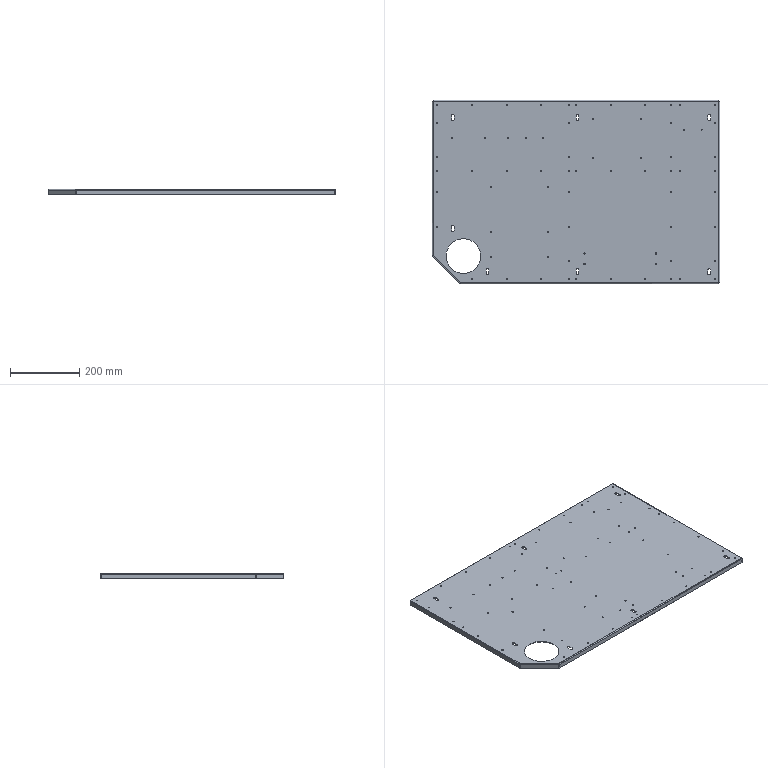Part | SolidWorks | features HoleWzd 2, BreakCorner 1, Cut 1, EdgeFlange 1, FlatPattern 1, SMBaseFlange 1, SheetMetal 1 | 1 solid | 221 faces | box 830 x 530 x 15 mm | volume 919562 mm3 | cylinder 170 | plane 41 | spline 10 | commonest cylinder face diameters 3.3 x144 8 x14 1.473 x5 5.473 x5 100 x2